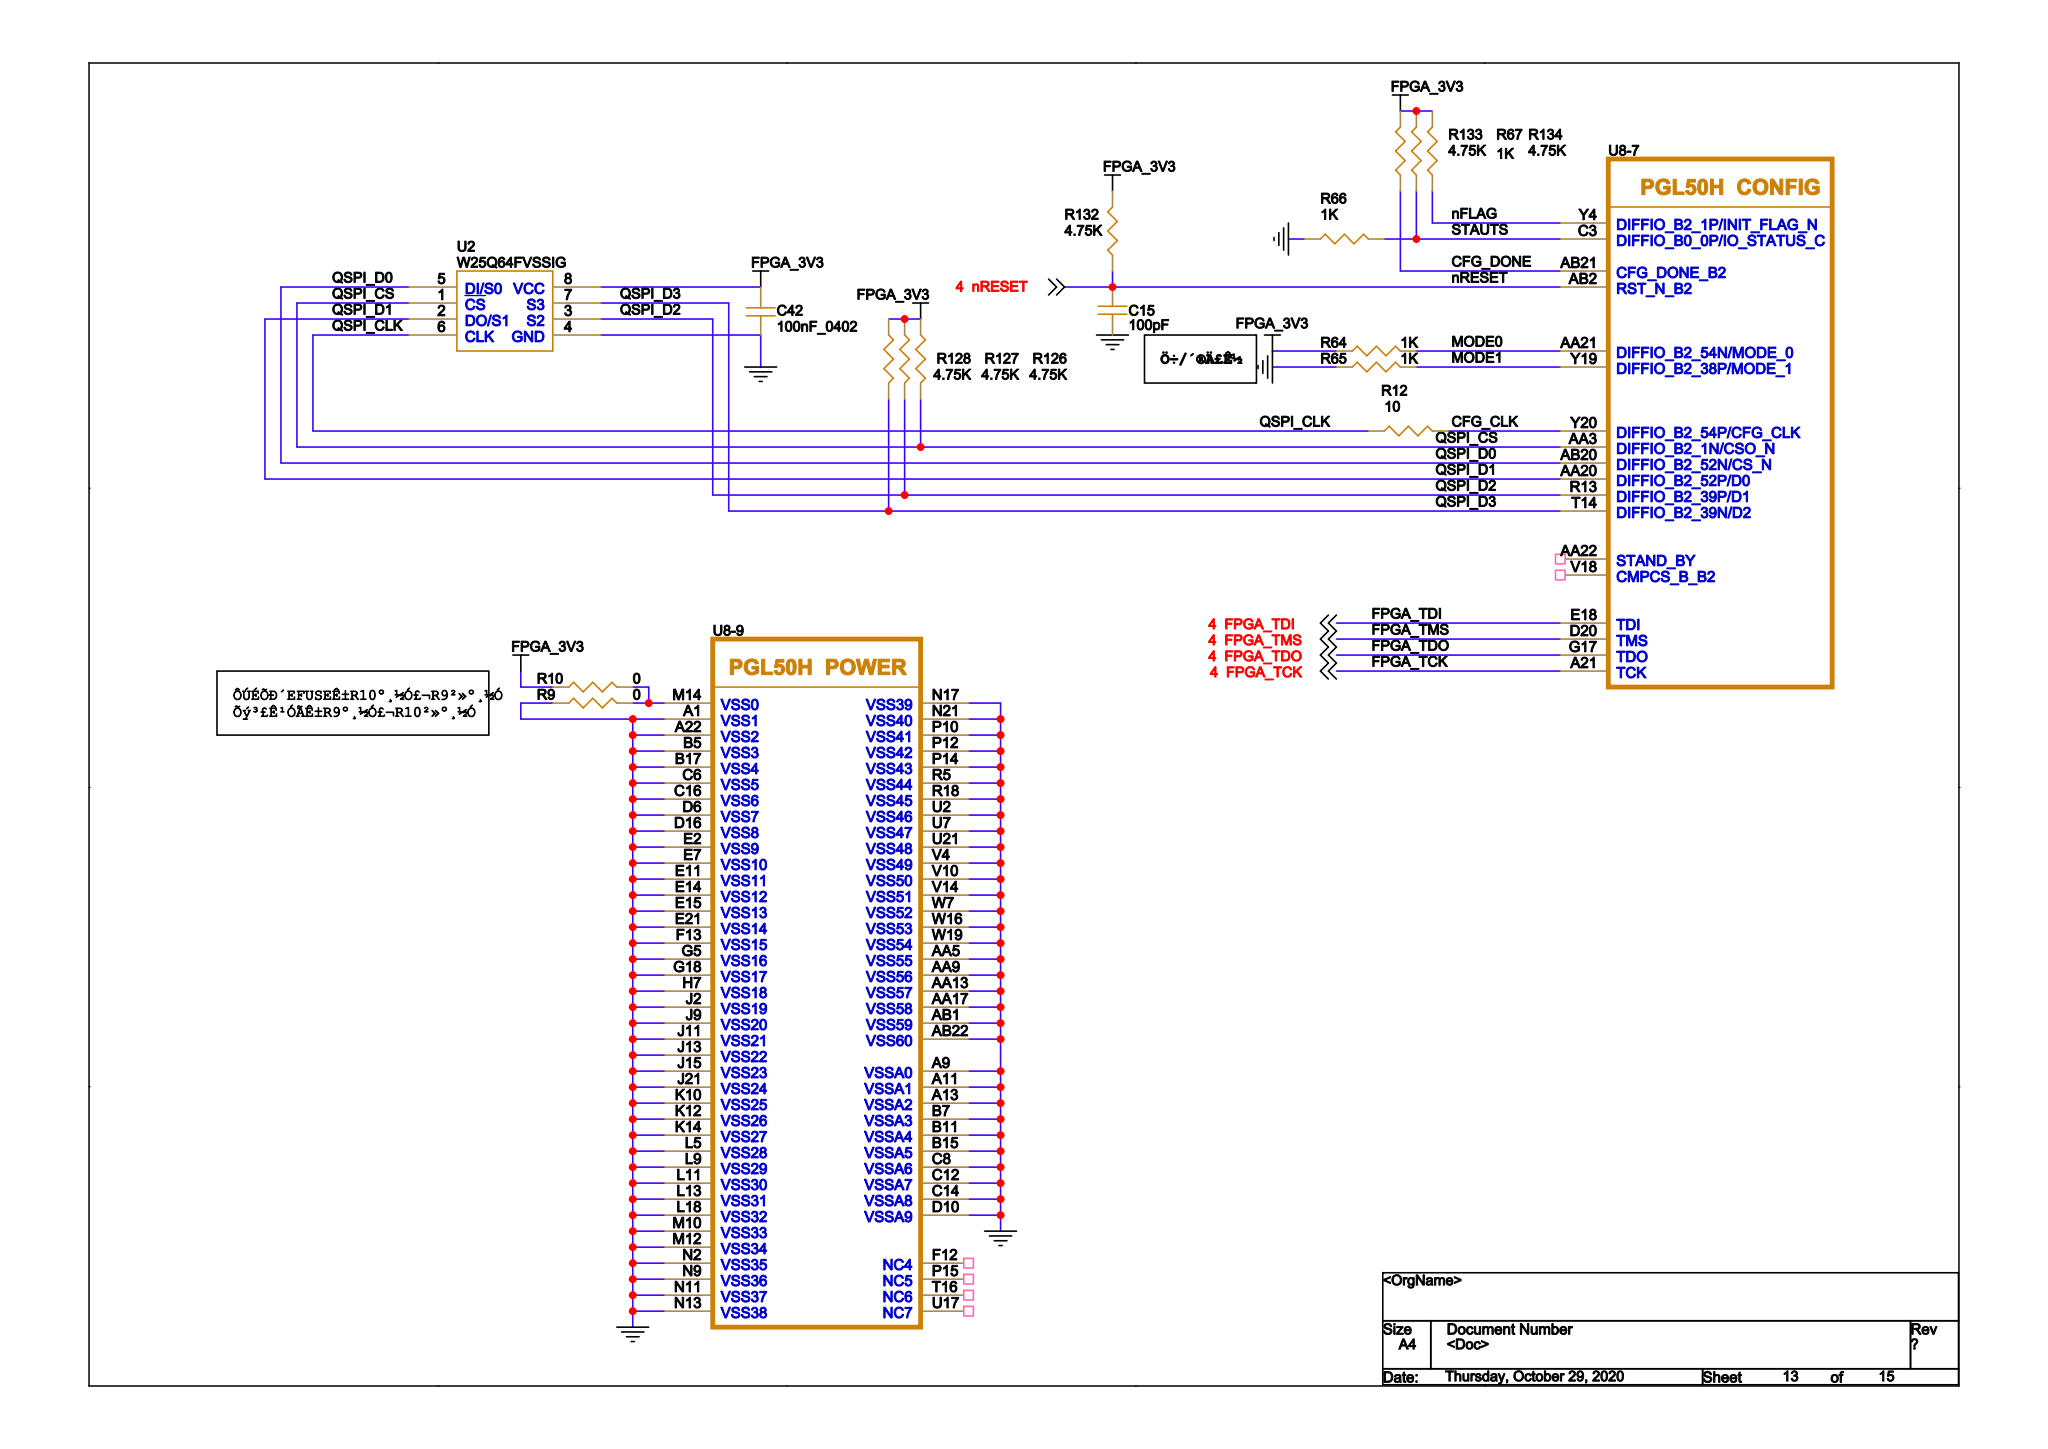Circuit board | Cadence Allegro | 406 parts | 392 nets | one sheet of the schematic
Parts on this sheet (reference | value | footprint):
C12 | 100pF | C_0603
C14 | 100pF | C_0603
C15 | 100pF | C_0603
C42 | 100nF_0402 | C_0402_104
R9 | 0 | R_0603
R12 | 10 | R_0603
R64 | 1K | R_0603
R65 | 1K | R_0603
R66 | 1K | R_0603
R67 | 1K | R_0603
R126 | 4.75K | R_0603
R127 | 4.75K | R_0603
R128 | 4.75K | R_0603
R132 | 4.75K | R_0603
R133 | 4.75K | R_0603
R134 | 4.75K | R_0603
U2 | W25Q64FVSSIG | U_SO8W
U17 | HXI15H4G160AF-13K | U_TFBGA96
Nets of these parts (net: part-pin ...):
GND: C12-2 C14-1 C15-2 C42-1 R9-1 R65-2 R66-2 U2-4 U17-A9 U17-E2 U17-J2
NRESET: C15-1 R132-1
FPGA_3V3: C42-2 R64-2 R67-1 R126-2 R127-2 R128-2 R132-2 R133-2 R134-2 U2-8
PHY_NRST: C12-1
DDR3_NREST: C14-2
N20313862: R9-2
CFG_CLK: R12-1
QSPI_CLK: R12-2 U2-6
QSPI_CS: R126-1 U2-1
QSPI_D2: R127-1 U2-3
QSPI_D3: R128-1 U2-7
CFG_DONE: R133-1
NFLAG: R134-1
MODE0: R64-1
MODE1: R65-1
STAUTS: R66-1 R67-2
QSPI_D0: U2-5
QSPI_D1: U2-2